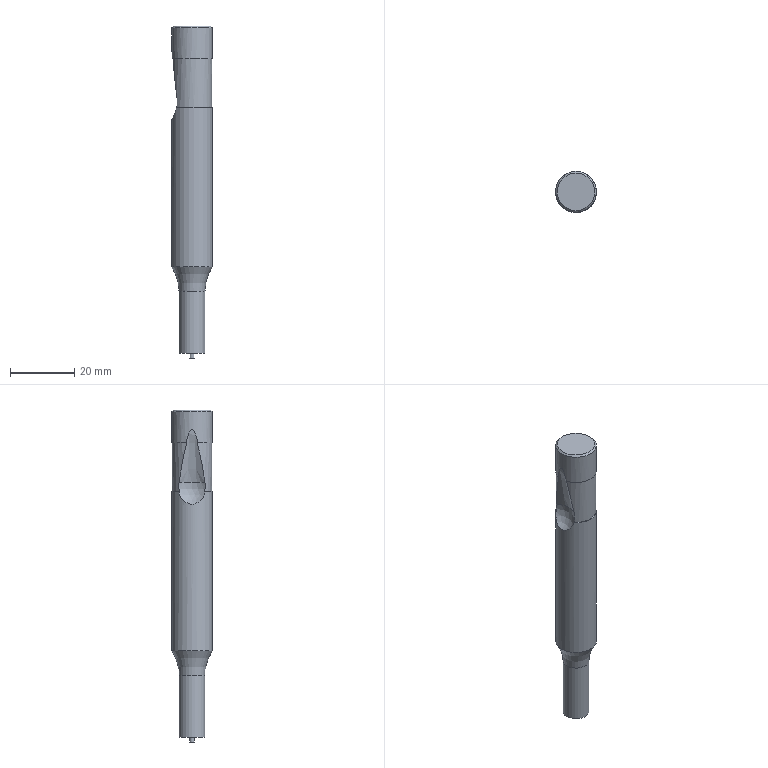Part | STEP file | 1_id482_x_t | 1 solid | 14 faces | box 12.7 x 12.7 x 103.124 mm | volume 10701 mm3 | plane 5 | cylinder 5 | cone 2 | torus 1 | sphere 1 | commonest cylinder face diameters 12.7 x2 1.473 x1 8.06 x1 12.294 x1